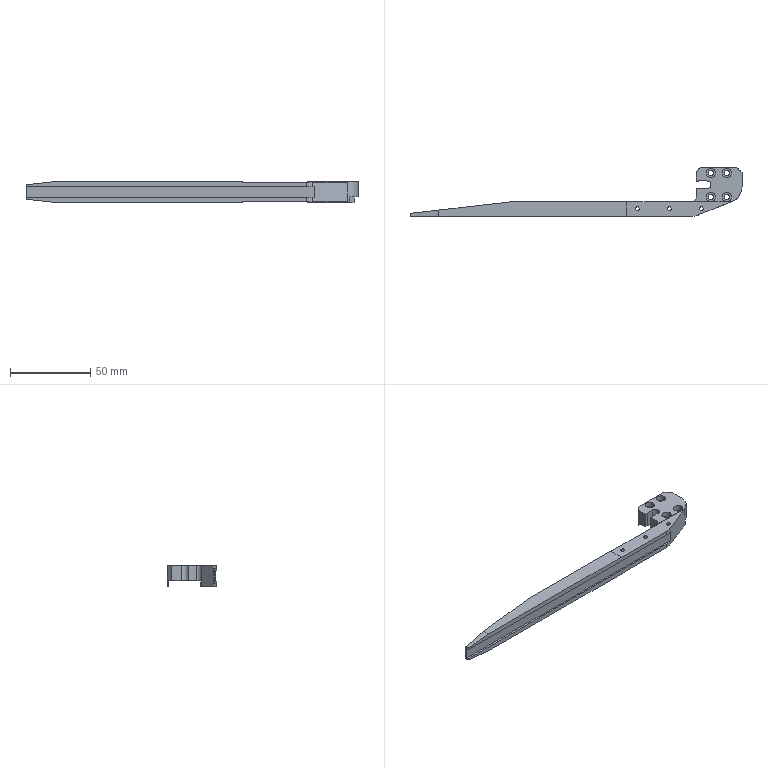NC program | NX | posted by the shop | part box 207.5 x 30.8 x 13 mm
Lines 3398 to 3456 of 6162:
N6 T07 M06
(D6-J  D=6. R=0. H=07 ce=0.30 di=0.00)
G00 G90 G54 X-53.313 Y-21.4 M03 S6000
G43 H07 Z20.
M08
Z.2
G01 Z-.3 F1200.
Y-16.
X-71.825
G02 X-75.761 Y-15.242 I.001 J10.6
G01 X-90.366 Y-9.4
X-72.25
G03 X-68.95 Y-6.1 I0.0 J3.3
X-69.005 Y-5.5 I-3.3 J0.0
G01 X-35.05
Y-16.
X-53.313
Y-11.8
X-67.376
X-71.988 Y-12.641
X-67.376 Y-11.8
G03 X-65.67 Y-9.7 I-4.874 J5.7
G01 X-39.25
Y-11.8
X-53.313
X-53.813
Y-21.4
Z.2
G00 Z20.
G00 G90 X-109.75 Y5.135 M03 S6000
Z20.
Z-2.9
G01 Z-3.4 F1200.
X-104.35
Y12.149
X-104.024 Y12.474
X-103.455 Y11.1
X-74.65
Y-2.3
X-100.789
X-101.22 Y-4.15
G02 X-104.35 Y3.37 I7.47 J7.52
G01 Y5.135
X-100.15
Y6.9
X-78.85
Y1.9
X-99.979
G02 X-100.15 Y3.37 I6.229 J1.47
G01 Y5.135
Y5.635
X-109.75
Z-2.9
G00 Z20.
G91 G28 Z0.0
M05
M09
G91 G28 Z0.0
M01